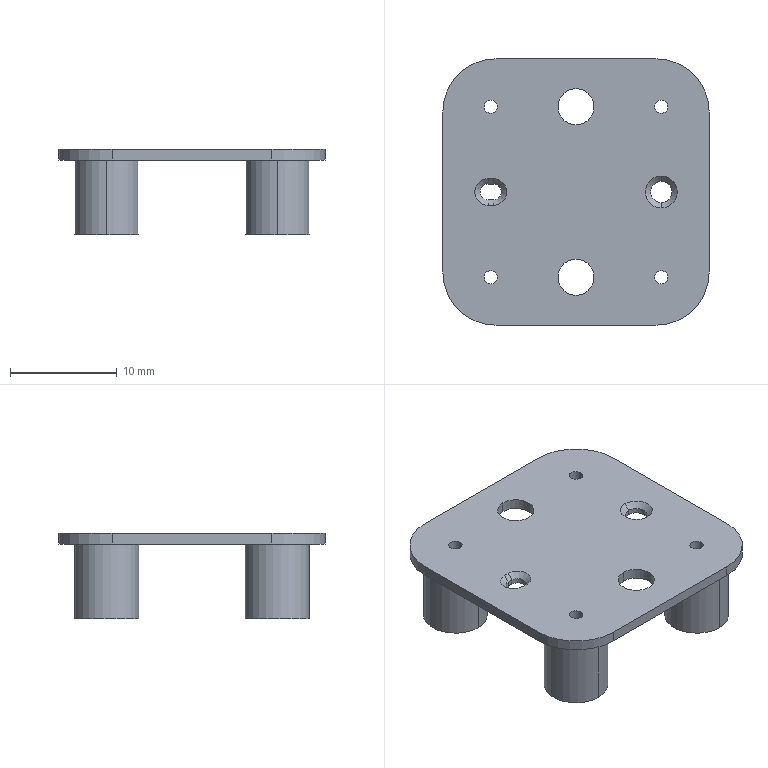Part | 1 solid | 74 faces | box 25 x 25 x 8 mm | volume 1312 mm3 | cylinder 36 | cone 20 | plane 18 | commonest cylinder face diameters 1.25 x8 2.2 x8 6 x8 3.4 x4 10 x4 1.5 x2